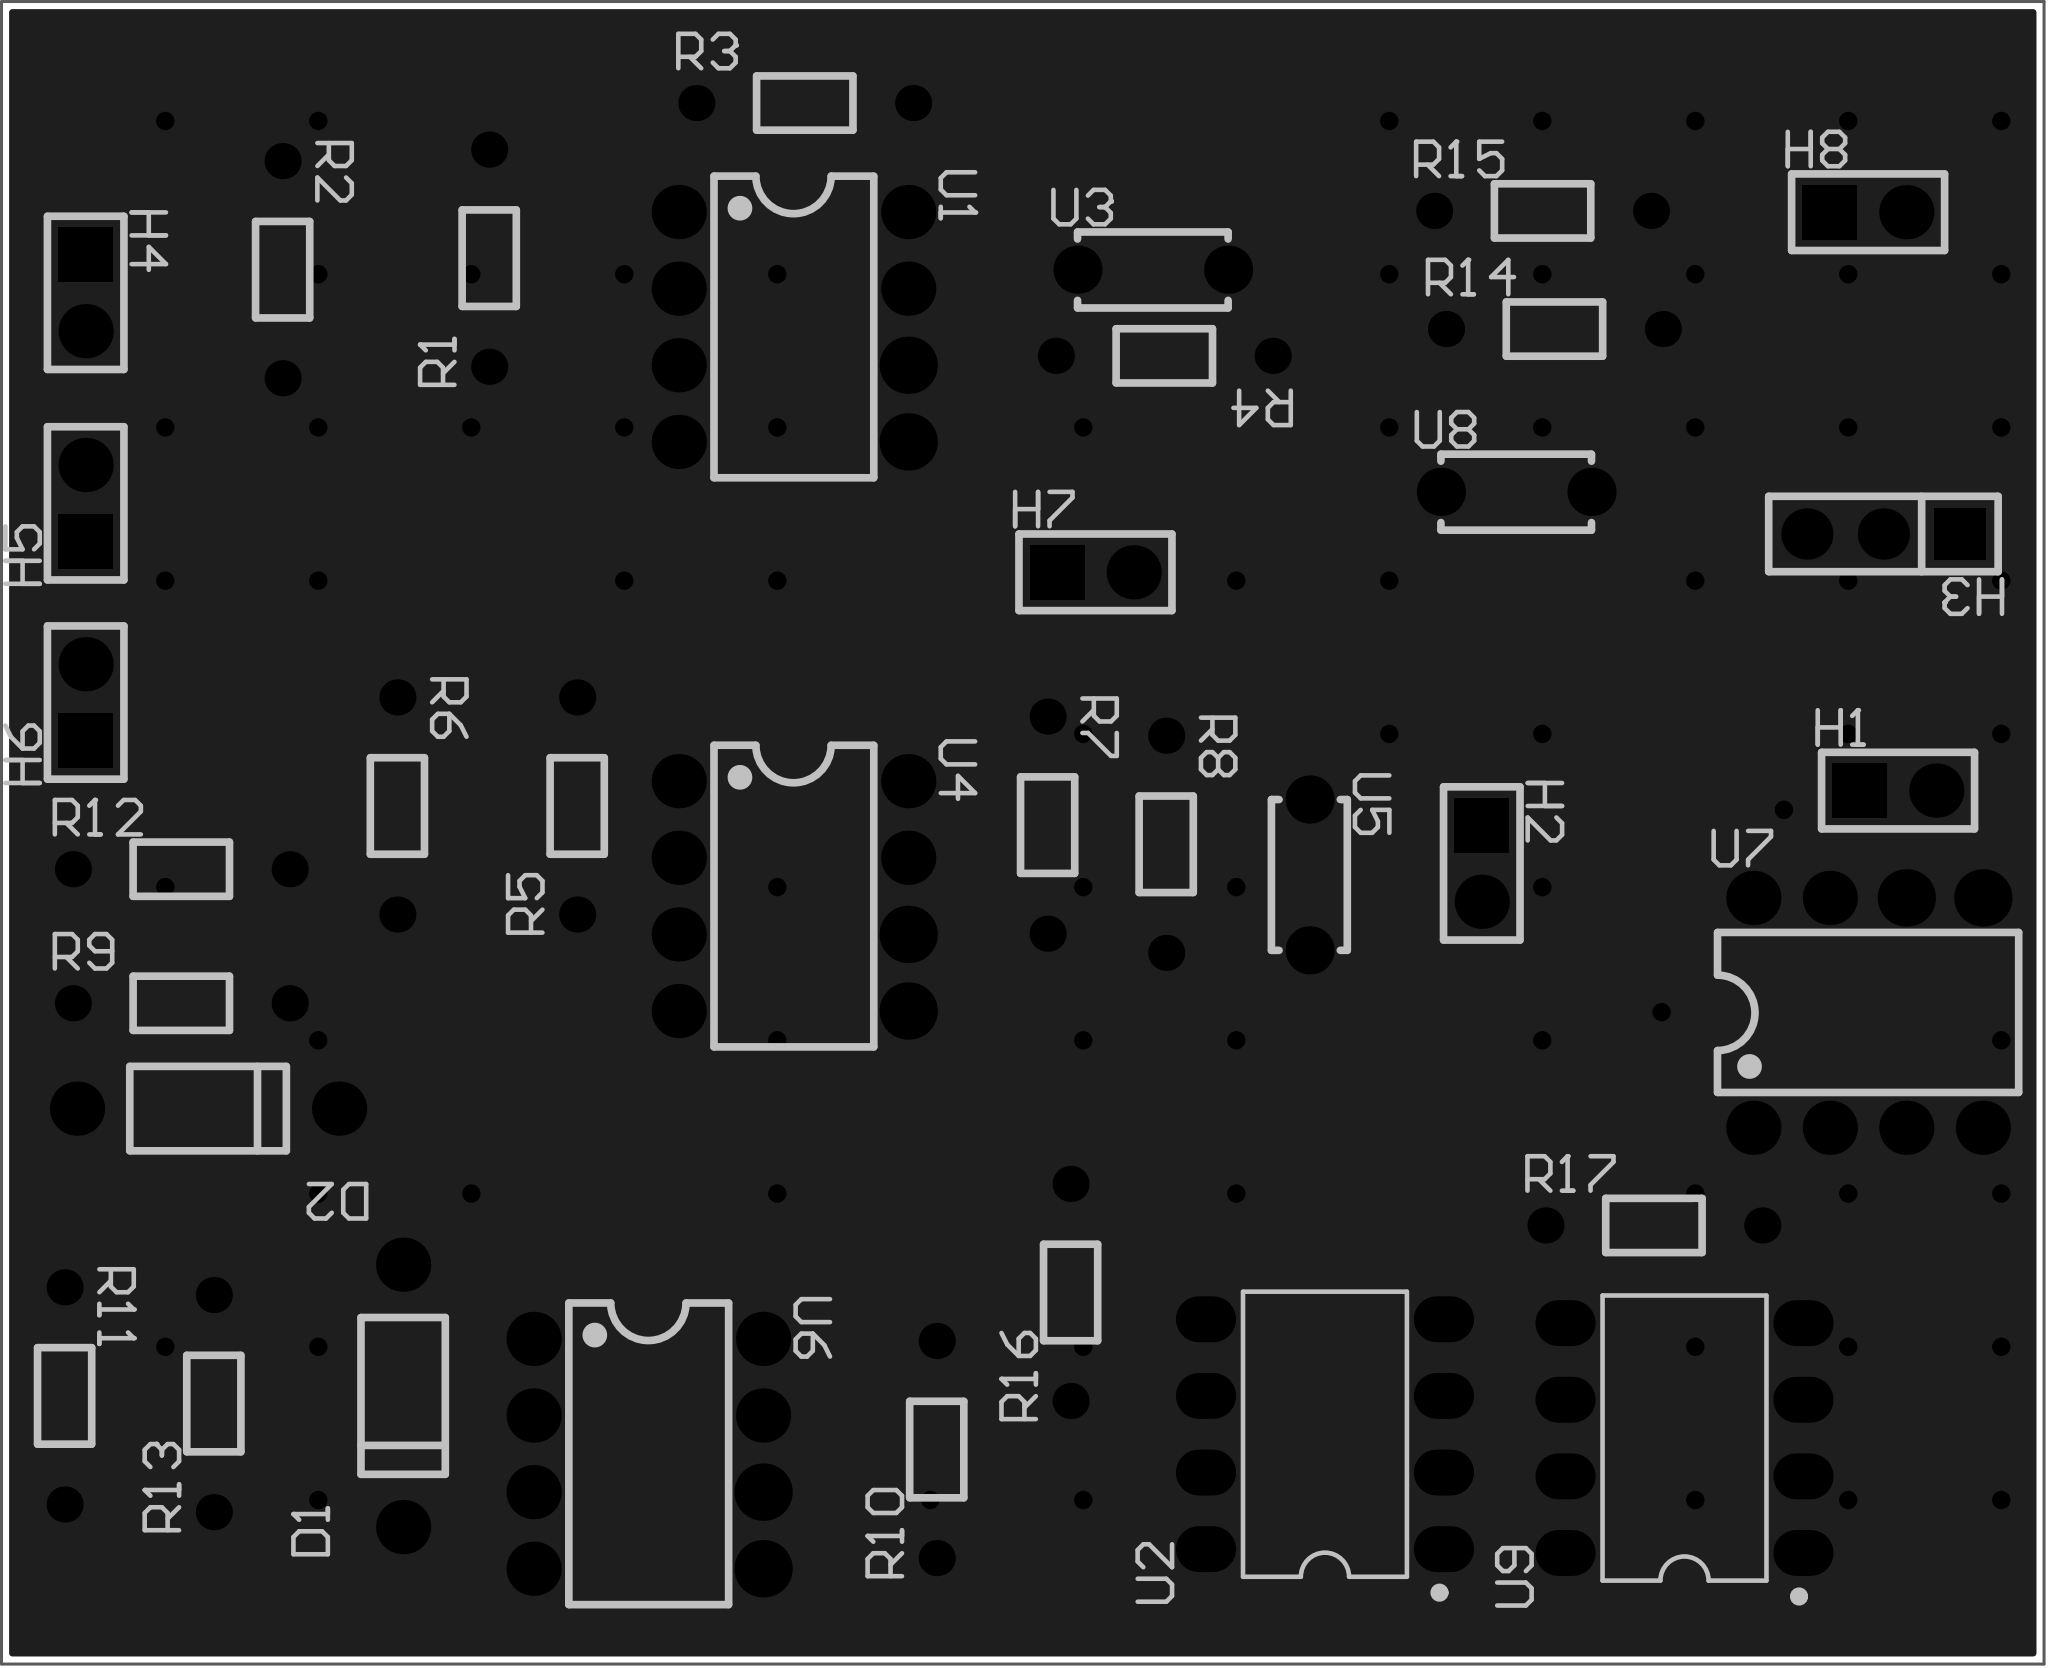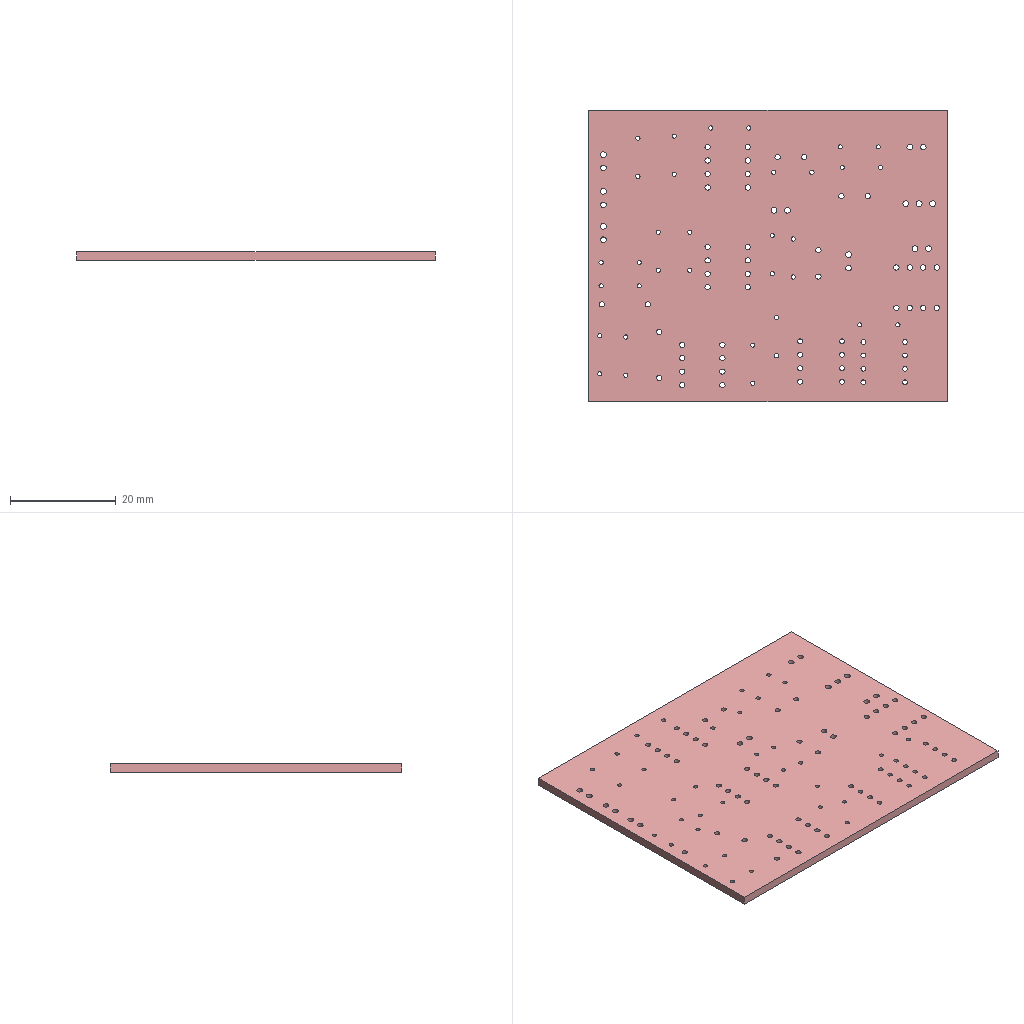Circuit board layout | Altium Designer | box 67.8 x 55.1 x 1.6 mm
Layer stack:
# Altium Designer layer stack of  (unit mm; dielectric type: 0 none, 1 core, 2 prepreg, 3 surface material)
index,name,kind,layer,copper_thickness_mm,dielectric_type,dielectric_thickness_mm,dielectric_material,dielectric_constant
0,Top Paste Mask Layer,other,,,,,,
1,Top Silkscreen Layer,other,,,,,,
2,Top Solder Mask Layer,dielectric,,,3,0.01,,3.3
3,Top Layer,copper,Top Layer,0.035,,,,
4,Dielectric1,dielectric,,,3,1.51,FR4,4.5
5,Bottom Layer,copper,Bottom Layer,0.035,,,,
6,Bottom Solder Mask Layer,dielectric,,,3,0.01,,3.3
7,Bottom Silkscreen Layer,other,,,,,,
8,Bottom Paste Mask Layer,other,,,,,,
# drill layer pairs: low layer,high layer
drill_pair,Top Layer,Bottom Layer
Part placement:
Designator,Comment,Layer,Footprint,Center-X(mm),Center-Y(mm),Rotation
D1,,TopLayer,DO_1N4007,97.663,90.805,90
D2,,TopLayer,DO_1N4007,91.186,100.33,180
H1,,TopLayer,HDR-TH_2P-P2.54-V-M-1,147.299,110.873,0
H2,,TopLayer,HDR-TH_2P-P2.54-V-M-1,133.477,108.458,270
H3,,TopLayer,HDR-TH_3P-P2.54-V-M,146.812,119.38,180
H4,,TopLayer,HDR-TH_2P-P2.54-V-M-1,87.122,127.375,270
H5,,TopLayer,HDR-TH_2P-P2.54-V-M-1,87.122,120.396,90
H6,,TopLayer,HDR-TH_2P-P2.54-V-M-1,87.122,113.792,90
H7,,TopLayer,HDR-TH_2P-P2.54-V-M-1,120.65,118.11,0
H8,,TopLayer,HDR-TH_2P-P2.54-V-M-1,146.304,130.048,0
R1,10kΩ,TopLayer,Res_1/8W,100.521,128.524,90
R2,10kΩ,TopLayer,Res_1/8W,93.662,128.143,270
R3,50kΩ,TopLayer,Res_1/8W,110.998,133.667,0
R4,18.1kΩ,TopLayer,Res_1/8W,122.936,125.286,180
R5,10kΩ,TopLayer,Res_1/8W,103.442,110.363,90
R6,10kΩ,TopLayer,Res_1/8W,97.472,110.363,270
R7,10kΩ,TopLayer,Res_1/8W,119.062,109.728,270
R8,40kΩ,TopLayer,Res_1/8W,122.999,109.093,270
R9,5kΩ,TopLayer,Res_1/8W,90.297,103.822,0
R10,10kΩ,TopLayer,Res_1/8W,115.38,89.027,90
R11,10kΩ,TopLayer,Res_1/8W,86.423,90.805,270
R12,10kΩ,TopLayer,Res_1/8W,90.297,108.267,0
R13,10kΩ,TopLayer,Res_1/8W,91.377,90.551,90
R14,71.68kΩ,TopLayer,Res_1/8W,135.89,126.174,0
R15,40kΩ,TopLayer,Res_1/8W,135.496,130.091,0
R16,567Ω,TopLayer,Res_1/8W,119.825,94.234,90
R17,2.67KΩ,TopLayer,Res_1/8W,139.192,96.456,0
U1,TL082CN(LX),TopLayer,PDIP-8_L9.6-W6.4-P2.54-LS7.6-BL,110.624,126.244,270
U2,AD633ANZ,TopLayer,PDIP-8_L9.3-W6.4-P2.54-LS7.9-BL-1,128.27,89.535,90
U3,10nF,TopLayer,CAP-TH_L5.0-W2.5-P5.00-D1.0,122.555,128.143,0
U4,TL082CN(LX),TopLayer,PDIP-8_L9.6-W6.4-P2.54-LS7.6-BL,110.624,107.376,270
U5,10nF,TopLayer,CAP-TH_L5.0-W2.5-P5.00-D1.0,127.762,108.077,270
U6,TL082CN(LX),TopLayer,PDIP-8_L9.6-W6.4-P2.54-LS7.6-BL,105.805,88.885,270
U7,TL082CN(LX),TopLayer,PDIP-8_L9.6-W6.4-P2.54-LS7.6-BL,146.304,103.505,0
U8,10nF,TopLayer,CAP-TH_L5.0-W2.5-P5.00-D1.0,134.62,120.777,0
U9,AD633ANZ,TopLayer,PDIP-8_L9.3-W6.4-P2.54-LS7.9-BL-1,140.208,89.408,90
Pad and via stacks:
# Altium Designer via and pad stacks of  (unit mm). Each distinct definition once, with the count of objects using it.
# via: kind,start_layer,end_layer,hole_mm,diameter_mm,mode(0 simple;1 top-mid-bottom;2 full stack),diameter_per_layer,count,example_net
# pad: kind,layer,hole_mm,hole_type(0 round;1 square;2 slot),plating,top_size,top_shape(1 round;2 rect;3 octagon;9 rounded rect),mid_size,bottom_size,mode,footprint,size_per_layer,count,example
pad,Multi-Layer,1,0,plated,1.8x1.8,1,1.8x1.8,1.8x1.8,0,DO_1N4007,,4,D1.1
pad,Multi-Layer,1.1,0,plated,1.8x1.8,1,1.8x1.8,1.8x1.8,0,HDR-TH_2P-P2.54-V-M-1,,7,H1.2
pad,Multi-Layer,1.1,0,plated,1.8x1.8,2,1.8x1.8,1.8x1.8,0,HDR-TH_2P-P2.54-V-M-1,,7,H1.1
pad,Multi-Layer,1.1,0,plated,1.7x1.7,2,1.7x1.7,1.7x1.7,0,HDR-TH_3P-P2.54-V-M,,1,H3.1
pad,Multi-Layer,1.1,0,plated,1.7x1.7,1,1.7x1.7,1.7x1.7,0,HDR-TH_3P-P2.54-V-M,,2,H3.2
pad,Multi-Layer,0.8001,0,plated,1.199x1.199,1,1.199x1.199,1.199x1.199,0,Res_1/8W,,34,R1.1
pad,Multi-Layer,1,0,plated,1.8x1.8,1,1.8x1.8,1.8x1.8,0,PDIP-8_L9.6-W6.4-P2.54-LS7.6-BL,,24,U1.1
pad,Multi-Layer,1,0,plated,1.905x1.905,1,1.905x1.905,1.905x1.905,0,PDIP-8_L9.6-W6.4-P2.54-LS7.6-BL,,8,U1.5
pad,Multi-Layer,0.9,0,plated,1.524x2,1,1.524x2,1.524x2,0,PDIP-8_L9.3-W6.4-P2.54-LS7.9-BL-1,,16,U2.1
pad,Multi-Layer,1,0,plated,1.6x1.6,1,1.6x1.6,1.6x1.6,0,CAP-TH_L5.0-W2.5-P5.00-D1.0,,6,U3.1
via,Top Layer,Bottom Layer,0.3048,0.61,0,,73,X
Copper pours:
name,layer,net,type(0 solid;1 hatched;2 none)
Bottom Layer-GND,Bottom Layer,GND,0
Top Layer-GND,Top Layer,GND,0
Design rules, without the lines most boards share:
# Altium Designer design rules of  (exported by Altium Designer, unit mm)
# columns: name | kind | enabled | priority | scope1 | scope2 | descriptor | typed fields (field=value)
creepage | 65 | enabled | 1 | All | All | Creepage Distance Constraint =(0mil) (All),(All) |
copperThickness1oz_2 | 2 | enabled | 2 | All | All | Width Constraint (Min=30mil) (Max=100mil) (Preferred=30mil) (All) |